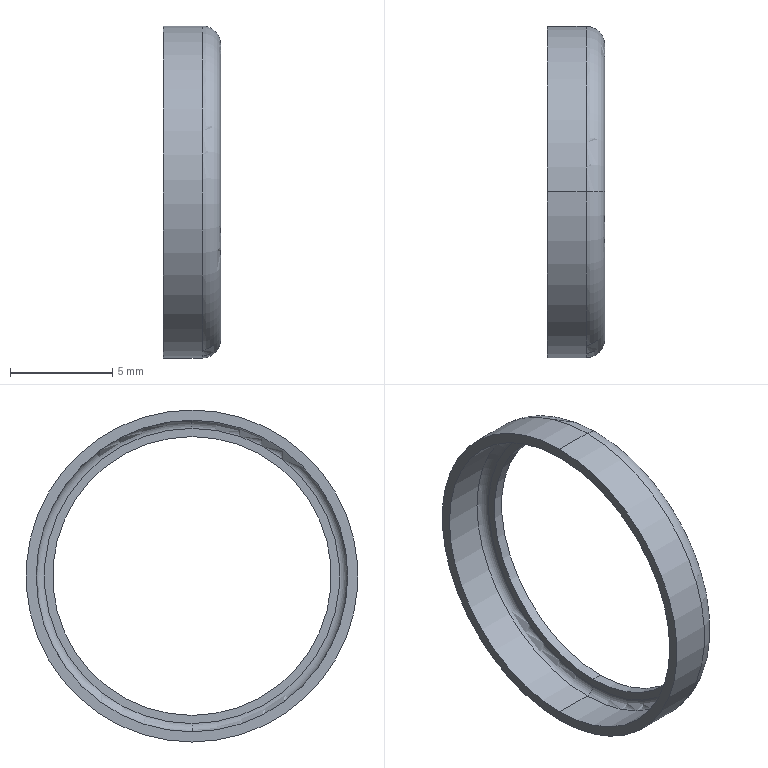Part | SolidWorks | features BaseBody 1 | 1 solid | 13 faces | box 2.8 x 16.2 x 16.2 mm | volume 80.141 mm3 | cylinder 6 | torus 4 | plane 3 | commonest cylinder face diameters 13.6 x2 15.2 x2 16.2 x2
STEP:
#1=CARTESIAN_POINT('',(0.03712,1.896,-204.65));
#2=VERTEX_POINT('',#1);
#3=CARTESIAN_POINT('',(0.03712,1.896,-188.45));
#4=VERTEX_POINT('',#3);
#5=CARTESIAN_POINT('',(0.03712,1.896,-196.55));
#6=DIRECTION('',(1.,0.,0.));
#7=DIRECTION('',(0.,0.,-1.));
#8=AXIS2_PLACEMENT_3D('',#5,#6,#7);
#9=CIRCLE('',#8,8.1);
#10=EDGE_CURVE('',#2,#4,#9,.T.);
#11=ORIENTED_EDGE('',*,*,#10,.T.);
#12=CARTESIAN_POINT('',(1.937,1.896,-188.45));
#13=VERTEX_POINT('',#12);
#14=CARTESIAN_POINT('',(2.837,1.896,-188.45));
#15=DIRECTION('',(1.,0.,0.));
#16=VECTOR('',#15,1000.);
#17=LINE('',#14,#16);
#18=EDGE_CURVE('',#4,#13,#17,.T.);
#19=ORIENTED_EDGE('',*,*,#18,.T.);
#20=CARTESIAN_POINT('',(1.937,1.896,-204.65));
#21=VERTEX_POINT('',#20);
#22=CARTESIAN_POINT('',(1.937,1.896,-196.55));
#23=DIRECTION('',(1.,0.,0.));
#24=DIRECTION('',(0.,0.,-1.));
#25=AXIS2_PLACEMENT_3D('',#22,#23,#24);
#26=CIRCLE('',#25,8.1);
#27=EDGE_CURVE('',#21,#13,#26,.T.);
#28=ORIENTED_EDGE('',*,*,#27,.F.);
#29=CARTESIAN_POINT('',(2.837,1.896,-204.65));
#30=DIRECTION('',(1.,0.,0.));
#31=VECTOR('',#30,1000.);
#32=LINE('',#29,#31);
#33=EDGE_CURVE('',#2,#21,#32,.T.);
#34=ORIENTED_EDGE('',*,*,#33,.F.);
#35=EDGE_LOOP('',(#11,#19,#28,#34));
#36=FACE_OUTER_BOUND('',#35,.T.);
#37=CARTESIAN_POINT('',(2.837,1.896,-196.55));
#38=DIRECTION('',(1.,0.,0.));
#39=DIRECTION('',(0.,0.,-1.));
#40=AXIS2_PLACEMENT_3D('',#37,#38,#39);
#41=CYLINDRICAL_SURFACE('',#40,8.1);
#42=ADVANCED_FACE('',(#36),#41,.T.);
#43=ORIENTED_EDGE('',*,*,#27,.T.);
#44=CARTESIAN_POINT('',(2.837,1.896,-189.35));
#45=VERTEX_POINT('',#44);
#46=CARTESIAN_POINT('',(1.937,1.896,-189.35));
#47=DIRECTION('',(0.,1.,0.));
#48=DIRECTION('',(-1.,0.,0.));
#49=AXIS2_PLACEMENT_3D('',#46,#47,#48);
#50=CIRCLE('',#49,0.9);
#51=EDGE_CURVE('',#13,#45,#50,.T.);
#52=ORIENTED_EDGE('',*,*,#51,.T.);
#53=CARTESIAN_POINT('',(2.837,1.896,-203.75));
#54=VERTEX_POINT('',#53);
#55=CARTESIAN_POINT('',(2.837,1.896,-196.55));
#56=DIRECTION('',(1.,0.,0.));
#57=DIRECTION('',(0.,0.,-1.));
#58=AXIS2_PLACEMENT_3D('',#55,#56,#57);
#59=CIRCLE('',#58,7.2);
#60=EDGE_CURVE('',#54,#45,#59,.T.);
#61=ORIENTED_EDGE('',*,*,#60,.F.);
#62=CARTESIAN_POINT('',(1.937,1.896,-203.75));
#63=DIRECTION('',(0.,-1.,0.));
#64=DIRECTION('',(1.,0.,0.));
#65=AXIS2_PLACEMENT_3D('',#62,#63,#64);
#66=CIRCLE('',#65,0.9);
#67=EDGE_CURVE('',#21,#54,#66,.T.);
#68=ORIENTED_EDGE('',*,*,#67,.F.);
#69=EDGE_LOOP('',(#43,#52,#61,#68));
#70=FACE_OUTER_BOUND('',#69,.T.);
#71=CARTESIAN_POINT('',(1.937,1.896,-196.55));
#72=DIRECTION('',(1.,0.,0.));
#73=DIRECTION('',(0.,0.,-1.));
#74=AXIS2_PLACEMENT_3D('',#71,#72,#73);
#75=TOROIDAL_SURFACE('',#74,7.2,0.9);
#76=ADVANCED_FACE('',(#70),#75,.T.);
#77=CARTESIAN_POINT('',(2.337,1.896,-189.75));
#78=VERTEX_POINT('',#77);
#79=CARTESIAN_POINT('',(2.337,1.896,-203.35));
#80=VERTEX_POINT('',#79);
#81=CARTESIAN_POINT('',(2.337,1.896,-196.55));
#82=DIRECTION('',(1.,0.,0.));
#83=DIRECTION('',(0.,0.,-1.));
#84=AXIS2_PLACEMENT_3D('',#81,#82,#83);
#85=CIRCLE('',#84,6.8);
#86=EDGE_CURVE('',#78,#80,#85,.T.);
#87=ORIENTED_EDGE('',*,*,#86,.F.);
#88=CARTESIAN_POINT('',(2.837,1.896,-189.75));
#89=VERTEX_POINT('',#88);
#90=CARTESIAN_POINT('',(2.837,1.896,-189.75));
#91=DIRECTION('',(1.,0.,0.));
#92=VECTOR('',#91,1000.);
#93=LINE('',#90,#92);
#94=EDGE_CURVE('',#78,#89,#93,.T.);
#95=ORIENTED_EDGE('',*,*,#94,.T.);
#96=CARTESIAN_POINT('',(2.837,1.896,-203.35));
#97=VERTEX_POINT('',#96);
#98=CARTESIAN_POINT('',(2.837,1.896,-196.55));
#99=DIRECTION('',(1.,0.,0.));
#100=DIRECTION('',(0.,0.,-1.));
#101=AXIS2_PLACEMENT_3D('',#98,#99,#100);
#102=CIRCLE('',#101,6.8);
#103=EDGE_CURVE('',#89,#97,#102,.T.);
#104=ORIENTED_EDGE('',*,*,#103,.T.);
#105=CARTESIAN_POINT('',(2.837,1.896,-203.35));
#106=DIRECTION('',(1.,0.,0.));
#107=VECTOR('',#106,1000.);
#108=LINE('',#105,#107);
#109=EDGE_CURVE('',#80,#97,#108,.T.);
#110=ORIENTED_EDGE('',*,*,#109,.F.);
#111=EDGE_LOOP('',(#87,#95,#104,#110));
#112=FACE_OUTER_BOUND('',#111,.T.);
#113=CARTESIAN_POINT('',(2.837,1.896,-196.55));
#114=DIRECTION('',(1.,0.,0.));
#115=DIRECTION('',(0.,0.,-1.));
#116=AXIS2_PLACEMENT_3D('',#113,#114,#115);
#117=CYLINDRICAL_SURFACE('',#116,6.8);
#118=ADVANCED_FACE('',(#112),#117,.F.);
#119=CARTESIAN_POINT('',(1.937,1.896,-188.95));
#120=VERTEX_POINT('',#119);
#121=CARTESIAN_POINT('',(1.937,1.896,-204.15));
#122=VERTEX_POINT('',#121);
#123=CARTESIAN_POINT('',(1.937,1.896,-196.55));
#124=DIRECTION('',(1.,0.,0.));
#125=DIRECTION('',(0.,0.,-1.));
#126=AXIS2_PLACEMENT_3D('',#123,#124,#125);
#127=CIRCLE('',#126,7.6);
#128=EDGE_CURVE('',#120,#122,#127,.T.);
#129=ORIENTED_EDGE('',*,*,#128,.F.);
#130=CARTESIAN_POINT('',(2.337,1.896,-189.35));
#131=VERTEX_POINT('',#130);
#132=CARTESIAN_POINT('',(1.937,1.896,-189.35));
#133=DIRECTION('',(0.,1.,0.));
#134=DIRECTION('',(-1.,0.,0.));
#135=AXIS2_PLACEMENT_3D('',#132,#133,#134);
#136=CIRCLE('',#135,0.4);
#137=EDGE_CURVE('',#120,#131,#136,.T.);
#138=ORIENTED_EDGE('',*,*,#137,.T.);
#139=CARTESIAN_POINT('',(2.337,1.896,-203.75));
#140=VERTEX_POINT('',#139);
#141=CARTESIAN_POINT('',(2.337,1.896,-196.55));
#142=DIRECTION('',(1.,0.,0.));
#143=DIRECTION('',(0.,0.,-1.));
#144=AXIS2_PLACEMENT_3D('',#141,#142,#143);
#145=CIRCLE('',#144,7.2);
#146=EDGE_CURVE('',#131,#140,#145,.T.);
#147=ORIENTED_EDGE('',*,*,#146,.T.);
#148=CARTESIAN_POINT('',(1.937,1.896,-203.75));
#149=DIRECTION('',(0.,-1.,0.));
#150=DIRECTION('',(1.,0.,0.));
#151=AXIS2_PLACEMENT_3D('',#148,#149,#150);
#152=CIRCLE('',#151,0.4);
#153=EDGE_CURVE('',#122,#140,#152,.T.);
#154=ORIENTED_EDGE('',*,*,#153,.F.);
#155=EDGE_LOOP('',(#129,#138,#147,#154));
#156=FACE_OUTER_BOUND('',#155,.T.);
#157=CARTESIAN_POINT('',(1.937,1.896,-196.55));
#158=DIRECTION('',(1.,0.,0.));
#159=DIRECTION('',(0.,0.,-1.));
#160=AXIS2_PLACEMENT_3D('',#157,#158,#159);
#161=TOROIDAL_SURFACE('',#160,7.2,0.4);
#162=ADVANCED_FACE('',(#156),#161,.F.);
#163=CARTESIAN_POINT('',(0.03712,1.896,-188.95));
#164=VERTEX_POINT('',#163);
#165=CARTESIAN_POINT('',(0.03712,1.896,-204.15));
#166=VERTEX_POINT('',#165);
#167=CARTESIAN_POINT('',(0.03712,1.896,-196.55));
#168=DIRECTION('',(1.,0.,0.));
#169=DIRECTION('',(0.,0.,-1.));
#170=AXIS2_PLACEMENT_3D('',#167,#168,#169);
#171=CIRCLE('',#170,7.6);
#172=EDGE_CURVE('',#164,#166,#171,.T.);
#173=ORIENTED_EDGE('',*,*,#172,.F.);
#174=CARTESIAN_POINT('',(2.837,1.896,-188.95));
#175=DIRECTION('',(1.,0.,0.));
#176=VECTOR('',#175,1000.);
#177=LINE('',#174,#176);
#178=EDGE_CURVE('',#164,#120,#177,.T.);
#179=ORIENTED_EDGE('',*,*,#178,.T.);
#180=ORIENTED_EDGE('',*,*,#128,.T.);
#181=CARTESIAN_POINT('',(2.837,1.896,-204.15));
#182=DIRECTION('',(1.,0.,0.));
#183=VECTOR('',#182,1000.);
#184=LINE('',#181,#183);
#185=EDGE_CURVE('',#166,#122,#184,.T.);
#186=ORIENTED_EDGE('',*,*,#185,.F.);
#187=EDGE_LOOP('',(#173,#179,#180,#186));
#188=FACE_OUTER_BOUND('',#187,.T.);
#189=CARTESIAN_POINT('',(2.837,1.896,-196.55));
#190=DIRECTION('',(1.,0.,0.));
#191=DIRECTION('',(0.,0.,-1.));
#192=AXIS2_PLACEMENT_3D('',#189,#190,#191);
#193=CYLINDRICAL_SURFACE('',#192,7.6);
#194=ADVANCED_FACE('',(#188),#193,.F.);
#195=ORIENTED_EDGE('',*,*,#178,.F.);
#196=CARTESIAN_POINT('',(0.03712,1.896,-196.55));
#197=DIRECTION('',(1.,0.,0.));
#198=DIRECTION('',(0.,0.,-1.));
#199=AXIS2_PLACEMENT_3D('',#196,#197,#198);
#200=CIRCLE('',#199,7.6);
#201=EDGE_CURVE('',#166,#164,#200,.T.);
#202=ORIENTED_EDGE('',*,*,#201,.F.);
#203=ORIENTED_EDGE('',*,*,#185,.T.);
#204=CARTESIAN_POINT('',(1.937,1.896,-196.55));
#205=DIRECTION('',(1.,0.,0.));
#206=DIRECTION('',(0.,0.,-1.));
#207=AXIS2_PLACEMENT_3D('',#204,#205,#206);
#208=CIRCLE('',#207,7.6);
#209=EDGE_CURVE('',#122,#120,#208,.T.);
#210=ORIENTED_EDGE('',*,*,#209,.T.);
#211=EDGE_LOOP('',(#195,#202,#203,#210));
#212=FACE_OUTER_BOUND('',#211,.T.);
#213=CARTESIAN_POINT('',(2.837,1.896,-196.55));
#214=DIRECTION('',(1.,0.,0.));
#215=DIRECTION('',(0.,0.,-1.));
#216=AXIS2_PLACEMENT_3D('',#213,#214,#215);
#217=CYLINDRICAL_SURFACE('',#216,7.6);
#218=ADVANCED_FACE('',(#212),#217,.F.);
#219=ORIENTED_EDGE('',*,*,#137,.F.);
#220=ORIENTED_EDGE('',*,*,#209,.F.);
#221=ORIENTED_EDGE('',*,*,#153,.T.);
#222=CARTESIAN_POINT('',(2.337,1.896,-196.55));
#223=DIRECTION('',(1.,0.,0.));
#224=DIRECTION('',(0.,0.,-1.));
#225=AXIS2_PLACEMENT_3D('',#222,#223,#224);
#226=CIRCLE('',#225,7.2);
#227=EDGE_CURVE('',#140,#131,#226,.T.);
#228=ORIENTED_EDGE('',*,*,#227,.T.);
#229=EDGE_LOOP('',(#219,#220,#221,#228));
#230=FACE_OUTER_BOUND('',#229,.T.);
#231=CARTESIAN_POINT('',(1.937,1.896,-196.55));
#232=DIRECTION('',(1.,0.,0.));
#233=DIRECTION('',(0.,0.,-1.));
#234=AXIS2_PLACEMENT_3D('',#231,#232,#233);
#235=TOROIDAL_SURFACE('',#234,7.2,0.4);
#236=ADVANCED_FACE('',(#230),#235,.F.);
#237=ORIENTED_EDGE('',*,*,#227,.F.);
#238=ORIENTED_EDGE('',*,*,#146,.F.);
#239=EDGE_LOOP('',(#237,#238));
#240=FACE_OUTER_BOUND('',#239,.T.);
#241=CARTESIAN_POINT('',(2.337,1.896,-196.55));
#242=DIRECTION('',(1.,0.,0.));
#243=DIRECTION('',(0.,0.,-1.));
#244=AXIS2_PLACEMENT_3D('',#241,#242,#243);
#245=CIRCLE('',#244,6.8);
#246=EDGE_CURVE('',#80,#78,#245,.T.);
#247=ORIENTED_EDGE('',*,*,#246,.T.);
#248=ORIENTED_EDGE('',*,*,#86,.T.);
#249=EDGE_LOOP('',(#247,#248));
#250=FACE_BOUND('',#249,.T.);
#251=CARTESIAN_POINT('',(2.337,9.096,-196.55));
#252=DIRECTION('',(-1.,0.,0.));
#253=DIRECTION('',(0.,1.,0.));
#254=AXIS2_PLACEMENT_3D('',#251,#252,#253);
#255=PLANE('',#254);
#256=ADVANCED_FACE('',(#240,#250),#255,.T.);
#257=ORIENTED_EDGE('',*,*,#94,.F.);
#258=ORIENTED_EDGE('',*,*,#246,.F.);
#259=ORIENTED_EDGE('',*,*,#109,.T.);
#260=CARTESIAN_POINT('',(2.837,1.896,-196.55));
#261=DIRECTION('',(1.,0.,0.));
#262=DIRECTION('',(0.,0.,-1.));
#263=AXIS2_PLACEMENT_3D('',#260,#261,#262);
#264=CIRCLE('',#263,6.8);
#265=EDGE_CURVE('',#97,#89,#264,.T.);
#266=ORIENTED_EDGE('',*,*,#265,.T.);
#267=EDGE_LOOP('',(#257,#258,#259,#266));
#268=FACE_OUTER_BOUND('',#267,.T.);
#269=CARTESIAN_POINT('',(2.837,1.896,-196.55));
#270=DIRECTION('',(1.,0.,0.));
#271=DIRECTION('',(0.,0.,-1.));
#272=AXIS2_PLACEMENT_3D('',#269,#270,#271);
#273=CYLINDRICAL_SURFACE('',#272,6.8);
#274=ADVANCED_FACE('',(#268),#273,.F.);
#275=ORIENTED_EDGE('',*,*,#265,.F.);
#276=ORIENTED_EDGE('',*,*,#103,.F.);
#277=EDGE_LOOP('',(#275,#276));
#278=FACE_BOUND('',#277,.T.);
#279=ORIENTED_EDGE('',*,*,#60,.T.);
#280=CARTESIAN_POINT('',(2.837,1.896,-196.55));
#281=DIRECTION('',(1.,0.,0.));
#282=DIRECTION('',(0.,0.,-1.));
#283=AXIS2_PLACEMENT_3D('',#280,#281,#282);
#284=CIRCLE('',#283,7.2);
#285=EDGE_CURVE('',#45,#54,#284,.T.);
#286=ORIENTED_EDGE('',*,*,#285,.T.);
#287=EDGE_LOOP('',(#279,#286));
#288=FACE_OUTER_BOUND('',#287,.T.);
#289=CARTESIAN_POINT('',(2.837,8.696,-196.55));
#290=DIRECTION('',(1.,0.,0.));
#291=DIRECTION('',(0.,1.,0.));
#292=AXIS2_PLACEMENT_3D('',#289,#290,#291);
#293=PLANE('',#292);
#294=ADVANCED_FACE('',(#278,#288),#293,.T.);
#295=ORIENTED_EDGE('',*,*,#51,.F.);
#296=CARTESIAN_POINT('',(1.937,1.896,-196.55));
#297=DIRECTION('',(1.,0.,0.));
#298=DIRECTION('',(0.,0.,-1.));
#299=AXIS2_PLACEMENT_3D('',#296,#297,#298);
#300=CIRCLE('',#299,8.1);
#301=EDGE_CURVE('',#13,#21,#300,.T.);
#302=ORIENTED_EDGE('',*,*,#301,.T.);
#303=ORIENTED_EDGE('',*,*,#67,.T.);
#304=ORIENTED_EDGE('',*,*,#285,.F.);
#305=EDGE_LOOP('',(#295,#302,#303,#304));
#306=FACE_OUTER_BOUND('',#305,.T.);
#307=CARTESIAN_POINT('',(1.937,1.896,-196.55));
#308=DIRECTION('',(1.,0.,0.));
#309=DIRECTION('',(0.,0.,-1.));
#310=AXIS2_PLACEMENT_3D('',#307,#308,#309);
#311=TOROIDAL_SURFACE('',#310,7.2,0.9);
#312=ADVANCED_FACE('',(#306),#311,.T.);
#313=ORIENTED_EDGE('',*,*,#18,.F.);
#314=CARTESIAN_POINT('',(0.03712,1.896,-196.55));
#315=DIRECTION('',(1.,0.,0.));
#316=DIRECTION('',(0.,0.,-1.));
#317=AXIS2_PLACEMENT_3D('',#314,#315,#316);
#318=CIRCLE('',#317,8.1);
#319=EDGE_CURVE('',#4,#2,#318,.T.);
#320=ORIENTED_EDGE('',*,*,#319,.T.);
#321=ORIENTED_EDGE('',*,*,#33,.T.);
#322=ORIENTED_EDGE('',*,*,#301,.F.);
#323=EDGE_LOOP('',(#313,#320,#321,#322));
#324=FACE_OUTER_BOUND('',#323,.T.);
#325=CARTESIAN_POINT('',(2.837,1.896,-196.55));
#326=DIRECTION('',(1.,0.,0.));
#327=DIRECTION('',(0.,0.,-1.));
#328=AXIS2_PLACEMENT_3D('',#325,#326,#327);
#329=CYLINDRICAL_SURFACE('',#328,8.1);
#330=ADVANCED_FACE('',(#324),#329,.T.);
#331=ORIENTED_EDGE('',*,*,#10,.F.);
#332=ORIENTED_EDGE('',*,*,#319,.F.);
#333=EDGE_LOOP('',(#331,#332));
#334=FACE_OUTER_BOUND('',#333,.T.);
#335=ORIENTED_EDGE('',*,*,#201,.T.);
#336=ORIENTED_EDGE('',*,*,#172,.T.);
#337=EDGE_LOOP('',(#335,#336));
#338=FACE_BOUND('',#337,.T.);
#339=CARTESIAN_POINT('',(0.03712,9.996,-196.55));
#340=DIRECTION('',(-1.,0.,0.));
#341=DIRECTION('',(0.,1.,0.));
#342=AXIS2_PLACEMENT_3D('',#339,#340,#341);
#343=PLANE('',#342);
#344=ADVANCED_FACE('',(#334,#338),#343,.T.);
#345=CLOSED_SHELL('',(#42,#76,#118,#162,#194,#218,#236,#256,#274,#294,#312,#330,#344));
#346=MANIFOLD_SOLID_BREP('',#345);
#347=CARTESIAN_POINT('',(0.,0.,0.));
#348=DIRECTION('',(0.,0.,1.));
#349=DIRECTION('',(1.,0.,0.));
#350=AXIS2_PLACEMENT_3D('',#347,#348,#349);
#351=(LENGTH_UNIT()NAMED_UNIT(*)SI_UNIT(.MILLI.,.METRE.));
#352=UNCERTAINTY_MEASURE_WITH_UNIT(LENGTH_MEASURE(0.00001),#351,'','');
#353=(NAMED_UNIT(*)PLANE_ANGLE_UNIT()SI_UNIT($,.RADIAN.));
#354=(NAMED_UNIT(*)SI_UNIT($,.STERADIAN.)SOLID_ANGLE_UNIT());
#355=(GEOMETRIC_REPRESENTATION_CONTEXT(3)GLOBAL_UNCERTAINTY_ASSIGNED_CONTEXT((#352))GLOBAL_UNIT_ASSIGNED_CONTEXT((#351,#353,#354))REPRESENTATION_CONTEXT('',''));
#356=ADVANCED_BREP_SHAPE_REPRESENTATION('',(#346,#350),#355);